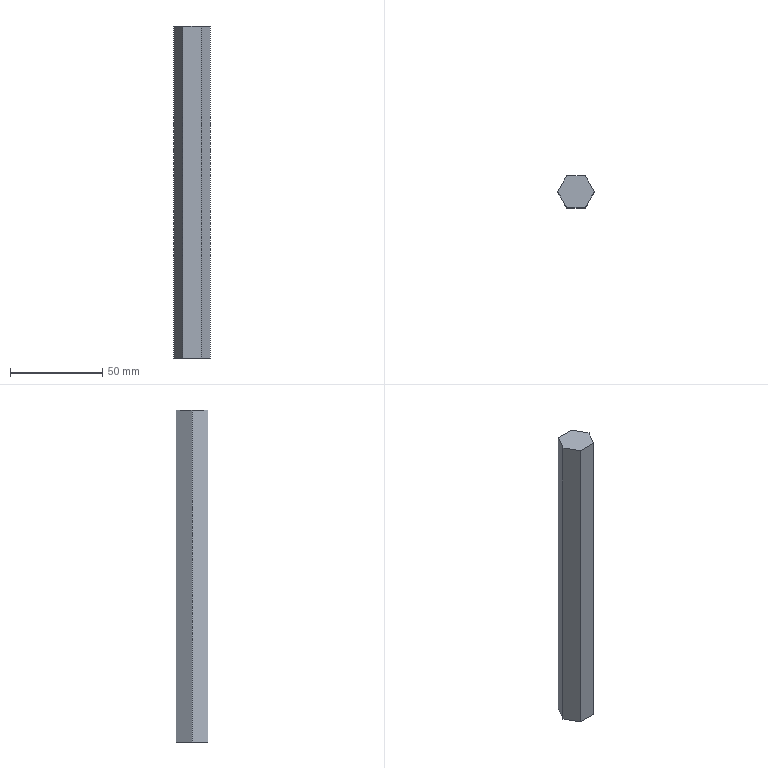Part | NX | 1 solid | 8 faces | box 20 x 17.321 x 180 mm | volume 46765 mm3 | plane 8
STEP:
#1=CARTESIAN_POINT('',(5.,-8.66,0.));
#2=VERTEX_POINT('',#1);
#3=CARTESIAN_POINT('',(10.,0.,0.));
#4=VERTEX_POINT('',#3);
#5=CARTESIAN_POINT('',(5.,-8.66,0.));
#6=DIRECTION('',(0.5,0.866,0.));
#7=VECTOR('',#6,1.);
#8=LINE('',#5,#7);
#9=EDGE_CURVE('',#2,#4,#8,.T.);
#10=ORIENTED_EDGE('',*,*,#9,.T.);
#11=CARTESIAN_POINT('',(10.,0.,180.));
#12=VERTEX_POINT('',#11);
#13=CARTESIAN_POINT('',(10.,0.,180.));
#14=DIRECTION('',(0.,0.,-1.));
#15=VECTOR('',#14,1.);
#16=LINE('',#13,#15);
#17=EDGE_CURVE('',#12,#4,#16,.T.);
#18=ORIENTED_EDGE('',*,*,#17,.F.);
#19=CARTESIAN_POINT('',(5.,-8.66,180.));
#20=VERTEX_POINT('',#19);
#21=CARTESIAN_POINT('',(5.,-8.66,180.));
#22=DIRECTION('',(0.5,0.866,0.));
#23=VECTOR('',#22,1.);
#24=LINE('',#21,#23);
#25=EDGE_CURVE('',#20,#12,#24,.T.);
#26=ORIENTED_EDGE('',*,*,#25,.F.);
#27=CARTESIAN_POINT('',(5.,-8.66,180.));
#28=DIRECTION('',(0.,0.,-1.));
#29=VECTOR('',#28,1.);
#30=LINE('',#27,#29);
#31=EDGE_CURVE('',#20,#2,#30,.T.);
#32=ORIENTED_EDGE('',*,*,#31,.T.);
#33=EDGE_LOOP('',(#10,#18,#26,#32));
#34=FACE_OUTER_BOUND('',#33,.T.);
#35=CARTESIAN_POINT('',(5.,-8.66,180.));
#36=DIRECTION('',(-0.866,0.5,0.));
#37=DIRECTION('',(-0.5,-0.866,0.));
#38=AXIS2_PLACEMENT_3D('',#35,#36,#37);
#39=PLANE('',#38);
#40=ADVANCED_FACE('',(#34),#39,.F.);
#41=CARTESIAN_POINT('',(5.,8.66,0.));
#42=VERTEX_POINT('',#41);
#43=CARTESIAN_POINT('',(10.,0.,0.));
#44=DIRECTION('',(-0.5,0.866,0.));
#45=VECTOR('',#44,1.);
#46=LINE('',#43,#45);
#47=EDGE_CURVE('',#4,#42,#46,.T.);
#48=ORIENTED_EDGE('',*,*,#47,.T.);
#49=CARTESIAN_POINT('',(5.,8.66,180.));
#50=VERTEX_POINT('',#49);
#51=CARTESIAN_POINT('',(5.,8.66,180.));
#52=DIRECTION('',(0.,0.,-1.));
#53=VECTOR('',#52,1.);
#54=LINE('',#51,#53);
#55=EDGE_CURVE('',#50,#42,#54,.T.);
#56=ORIENTED_EDGE('',*,*,#55,.F.);
#57=CARTESIAN_POINT('',(10.,0.,180.));
#58=DIRECTION('',(-0.5,0.866,0.));
#59=VECTOR('',#58,1.);
#60=LINE('',#57,#59);
#61=EDGE_CURVE('',#12,#50,#60,.T.);
#62=ORIENTED_EDGE('',*,*,#61,.F.);
#63=ORIENTED_EDGE('',*,*,#17,.T.);
#64=EDGE_LOOP('',(#48,#56,#62,#63));
#65=FACE_OUTER_BOUND('',#64,.T.);
#66=CARTESIAN_POINT('',(10.,0.,180.));
#67=DIRECTION('',(-0.866,-0.5,0.));
#68=DIRECTION('',(0.5,-0.866,0.));
#69=AXIS2_PLACEMENT_3D('',#66,#67,#68);
#70=PLANE('',#69);
#71=ADVANCED_FACE('',(#65),#70,.F.);
#72=CARTESIAN_POINT('',(-5.,8.66,0.));
#73=VERTEX_POINT('',#72);
#74=CARTESIAN_POINT('',(5.,8.66,0.));
#75=DIRECTION('',(-1.,0.,0.));
#76=VECTOR('',#75,1.);
#77=LINE('',#74,#76);
#78=EDGE_CURVE('',#42,#73,#77,.T.);
#79=ORIENTED_EDGE('',*,*,#78,.T.);
#80=CARTESIAN_POINT('',(-5.,8.66,180.));
#81=VERTEX_POINT('',#80);
#82=CARTESIAN_POINT('',(-5.,8.66,180.));
#83=DIRECTION('',(0.,0.,-1.));
#84=VECTOR('',#83,1.);
#85=LINE('',#82,#84);
#86=EDGE_CURVE('',#81,#73,#85,.T.);
#87=ORIENTED_EDGE('',*,*,#86,.F.);
#88=CARTESIAN_POINT('',(5.,8.66,180.));
#89=DIRECTION('',(-1.,0.,0.));
#90=VECTOR('',#89,1.);
#91=LINE('',#88,#90);
#92=EDGE_CURVE('',#50,#81,#91,.T.);
#93=ORIENTED_EDGE('',*,*,#92,.F.);
#94=ORIENTED_EDGE('',*,*,#55,.T.);
#95=EDGE_LOOP('',(#79,#87,#93,#94));
#96=FACE_OUTER_BOUND('',#95,.T.);
#97=CARTESIAN_POINT('',(5.,8.66,180.));
#98=DIRECTION('',(0.,-1.,0.));
#99=DIRECTION('',(1.,0.,0.));
#100=AXIS2_PLACEMENT_3D('',#97,#98,#99);
#101=PLANE('',#100);
#102=ADVANCED_FACE('',(#96),#101,.F.);
#103=CARTESIAN_POINT('',(-10.,0.,0.));
#104=VERTEX_POINT('',#103);
#105=CARTESIAN_POINT('',(-5.,8.66,0.));
#106=DIRECTION('',(-0.5,-0.866,0.));
#107=VECTOR('',#106,1.);
#108=LINE('',#105,#107);
#109=EDGE_CURVE('',#73,#104,#108,.T.);
#110=ORIENTED_EDGE('',*,*,#109,.T.);
#111=CARTESIAN_POINT('',(-10.,0.,180.));
#112=VERTEX_POINT('',#111);
#113=CARTESIAN_POINT('',(-10.,0.,180.));
#114=DIRECTION('',(0.,0.,-1.));
#115=VECTOR('',#114,1.);
#116=LINE('',#113,#115);
#117=EDGE_CURVE('',#112,#104,#116,.T.);
#118=ORIENTED_EDGE('',*,*,#117,.F.);
#119=CARTESIAN_POINT('',(-5.,8.66,180.));
#120=DIRECTION('',(-0.5,-0.866,0.));
#121=VECTOR('',#120,1.);
#122=LINE('',#119,#121);
#123=EDGE_CURVE('',#81,#112,#122,.T.);
#124=ORIENTED_EDGE('',*,*,#123,.F.);
#125=ORIENTED_EDGE('',*,*,#86,.T.);
#126=EDGE_LOOP('',(#110,#118,#124,#125));
#127=FACE_OUTER_BOUND('',#126,.T.);
#128=CARTESIAN_POINT('',(-5.,8.66,180.));
#129=DIRECTION('',(0.866,-0.5,0.));
#130=DIRECTION('',(0.5,0.866,0.));
#131=AXIS2_PLACEMENT_3D('',#128,#129,#130);
#132=PLANE('',#131);
#133=ADVANCED_FACE('',(#127),#132,.F.);
#134=CARTESIAN_POINT('',(-5.,-8.66,0.));
#135=VERTEX_POINT('',#134);
#136=CARTESIAN_POINT('',(-10.,0.,0.));
#137=DIRECTION('',(0.5,-0.866,0.));
#138=VECTOR('',#137,1.);
#139=LINE('',#136,#138);
#140=EDGE_CURVE('',#104,#135,#139,.T.);
#141=ORIENTED_EDGE('',*,*,#140,.T.);
#142=CARTESIAN_POINT('',(-5.,-8.66,180.));
#143=VERTEX_POINT('',#142);
#144=CARTESIAN_POINT('',(-5.,-8.66,180.));
#145=DIRECTION('',(0.,0.,-1.));
#146=VECTOR('',#145,1.);
#147=LINE('',#144,#146);
#148=EDGE_CURVE('',#143,#135,#147,.T.);
#149=ORIENTED_EDGE('',*,*,#148,.F.);
#150=CARTESIAN_POINT('',(-10.,0.,180.));
#151=DIRECTION('',(0.5,-0.866,0.));
#152=VECTOR('',#151,1.);
#153=LINE('',#150,#152);
#154=EDGE_CURVE('',#112,#143,#153,.T.);
#155=ORIENTED_EDGE('',*,*,#154,.F.);
#156=ORIENTED_EDGE('',*,*,#117,.T.);
#157=EDGE_LOOP('',(#141,#149,#155,#156));
#158=FACE_OUTER_BOUND('',#157,.T.);
#159=CARTESIAN_POINT('',(-10.,0.,180.));
#160=DIRECTION('',(0.866,0.5,0.));
#161=DIRECTION('',(-0.5,0.866,0.));
#162=AXIS2_PLACEMENT_3D('',#159,#160,#161);
#163=PLANE('',#162);
#164=ADVANCED_FACE('',(#158),#163,.F.);
#165=CARTESIAN_POINT('',(-5.,-8.66,0.));
#166=DIRECTION('',(1.,0.,0.));
#167=VECTOR('',#166,1.);
#168=LINE('',#165,#167);
#169=EDGE_CURVE('',#135,#2,#168,.T.);
#170=ORIENTED_EDGE('',*,*,#169,.T.);
#171=ORIENTED_EDGE('',*,*,#31,.F.);
#172=CARTESIAN_POINT('',(-5.,-8.66,180.));
#173=DIRECTION('',(1.,0.,0.));
#174=VECTOR('',#173,1.);
#175=LINE('',#172,#174);
#176=EDGE_CURVE('',#143,#20,#175,.T.);
#177=ORIENTED_EDGE('',*,*,#176,.F.);
#178=ORIENTED_EDGE('',*,*,#148,.T.);
#179=EDGE_LOOP('',(#170,#171,#177,#178));
#180=FACE_OUTER_BOUND('',#179,.T.);
#181=CARTESIAN_POINT('',(-5.,-8.66,180.));
#182=DIRECTION('',(0.,1.,0.));
#183=DIRECTION('',(-1.,0.,0.));
#184=AXIS2_PLACEMENT_3D('',#181,#182,#183);
#185=PLANE('',#184);
#186=ADVANCED_FACE('',(#180),#185,.F.);
#187=ORIENTED_EDGE('',*,*,#25,.T.);
#188=ORIENTED_EDGE('',*,*,#61,.T.);
#189=ORIENTED_EDGE('',*,*,#92,.T.);
#190=ORIENTED_EDGE('',*,*,#123,.T.);
#191=ORIENTED_EDGE('',*,*,#154,.T.);
#192=ORIENTED_EDGE('',*,*,#176,.T.);
#193=EDGE_LOOP('',(#187,#188,#189,#190,#191,#192));
#194=FACE_OUTER_BOUND('',#193,.T.);
#195=CARTESIAN_POINT('',(10.,0.,180.));
#196=DIRECTION('',(0.,0.,1.));
#197=DIRECTION('',(1.,0.,0.));
#198=AXIS2_PLACEMENT_3D('',#195,#196,#197);
#199=PLANE('',#198);
#200=ADVANCED_FACE('',(#194),#199,.T.);
#201=ORIENTED_EDGE('',*,*,#9,.F.);
#202=ORIENTED_EDGE('',*,*,#169,.F.);
#203=ORIENTED_EDGE('',*,*,#140,.F.);
#204=ORIENTED_EDGE('',*,*,#109,.F.);
#205=ORIENTED_EDGE('',*,*,#78,.F.);
#206=ORIENTED_EDGE('',*,*,#47,.F.);
#207=EDGE_LOOP('',(#201,#202,#203,#204,#205,#206));
#208=FACE_OUTER_BOUND('',#207,.T.);
#209=CARTESIAN_POINT('',(10.,0.,0.));
#210=DIRECTION('',(0.,0.,1.));
#211=DIRECTION('',(1.,0.,0.));
#212=AXIS2_PLACEMENT_3D('',#209,#210,#211);
#213=PLANE('',#212);
#214=ADVANCED_FACE('',(#208),#213,.F.);
#215=CLOSED_SHELL('',(#40,#71,#102,#133,#164,#186,#200,#214));
#216=MANIFOLD_SOLID_BREP('',#215);
#217=(LENGTH_UNIT()NAMED_UNIT(*)SI_UNIT(.MILLI.,.METRE.));
#218=UNCERTAINTY_MEASURE_WITH_UNIT(LENGTH_MEASURE(0.00002),#217,'','');
#219=(NAMED_UNIT(*)PLANE_ANGLE_UNIT()SI_UNIT($,.RADIAN.));
#220=PLANE_ANGLE_MEASURE_WITH_UNIT(PLANE_ANGLE_MEASURE(0.01745),#219);
#221=DIMENSIONAL_EXPONENTS(0.,0.,0.,0.,0.,0.,0.);
#222=(CONVERSION_BASED_UNIT('DEGREE',#220)NAMED_UNIT(#221)PLANE_ANGLE_UNIT());
#223=(NAMED_UNIT(*)SI_UNIT($,.STERADIAN.)SOLID_ANGLE_UNIT());
#224=(GEOMETRIC_REPRESENTATION_CONTEXT(3)GLOBAL_UNCERTAINTY_ASSIGNED_CONTEXT((#218))GLOBAL_UNIT_ASSIGNED_CONTEXT((#217,#222,#223))REPRESENTATION_CONTEXT('',''));
#225=ADVANCED_BREP_SHAPE_REPRESENTATION('',(#216),#224);